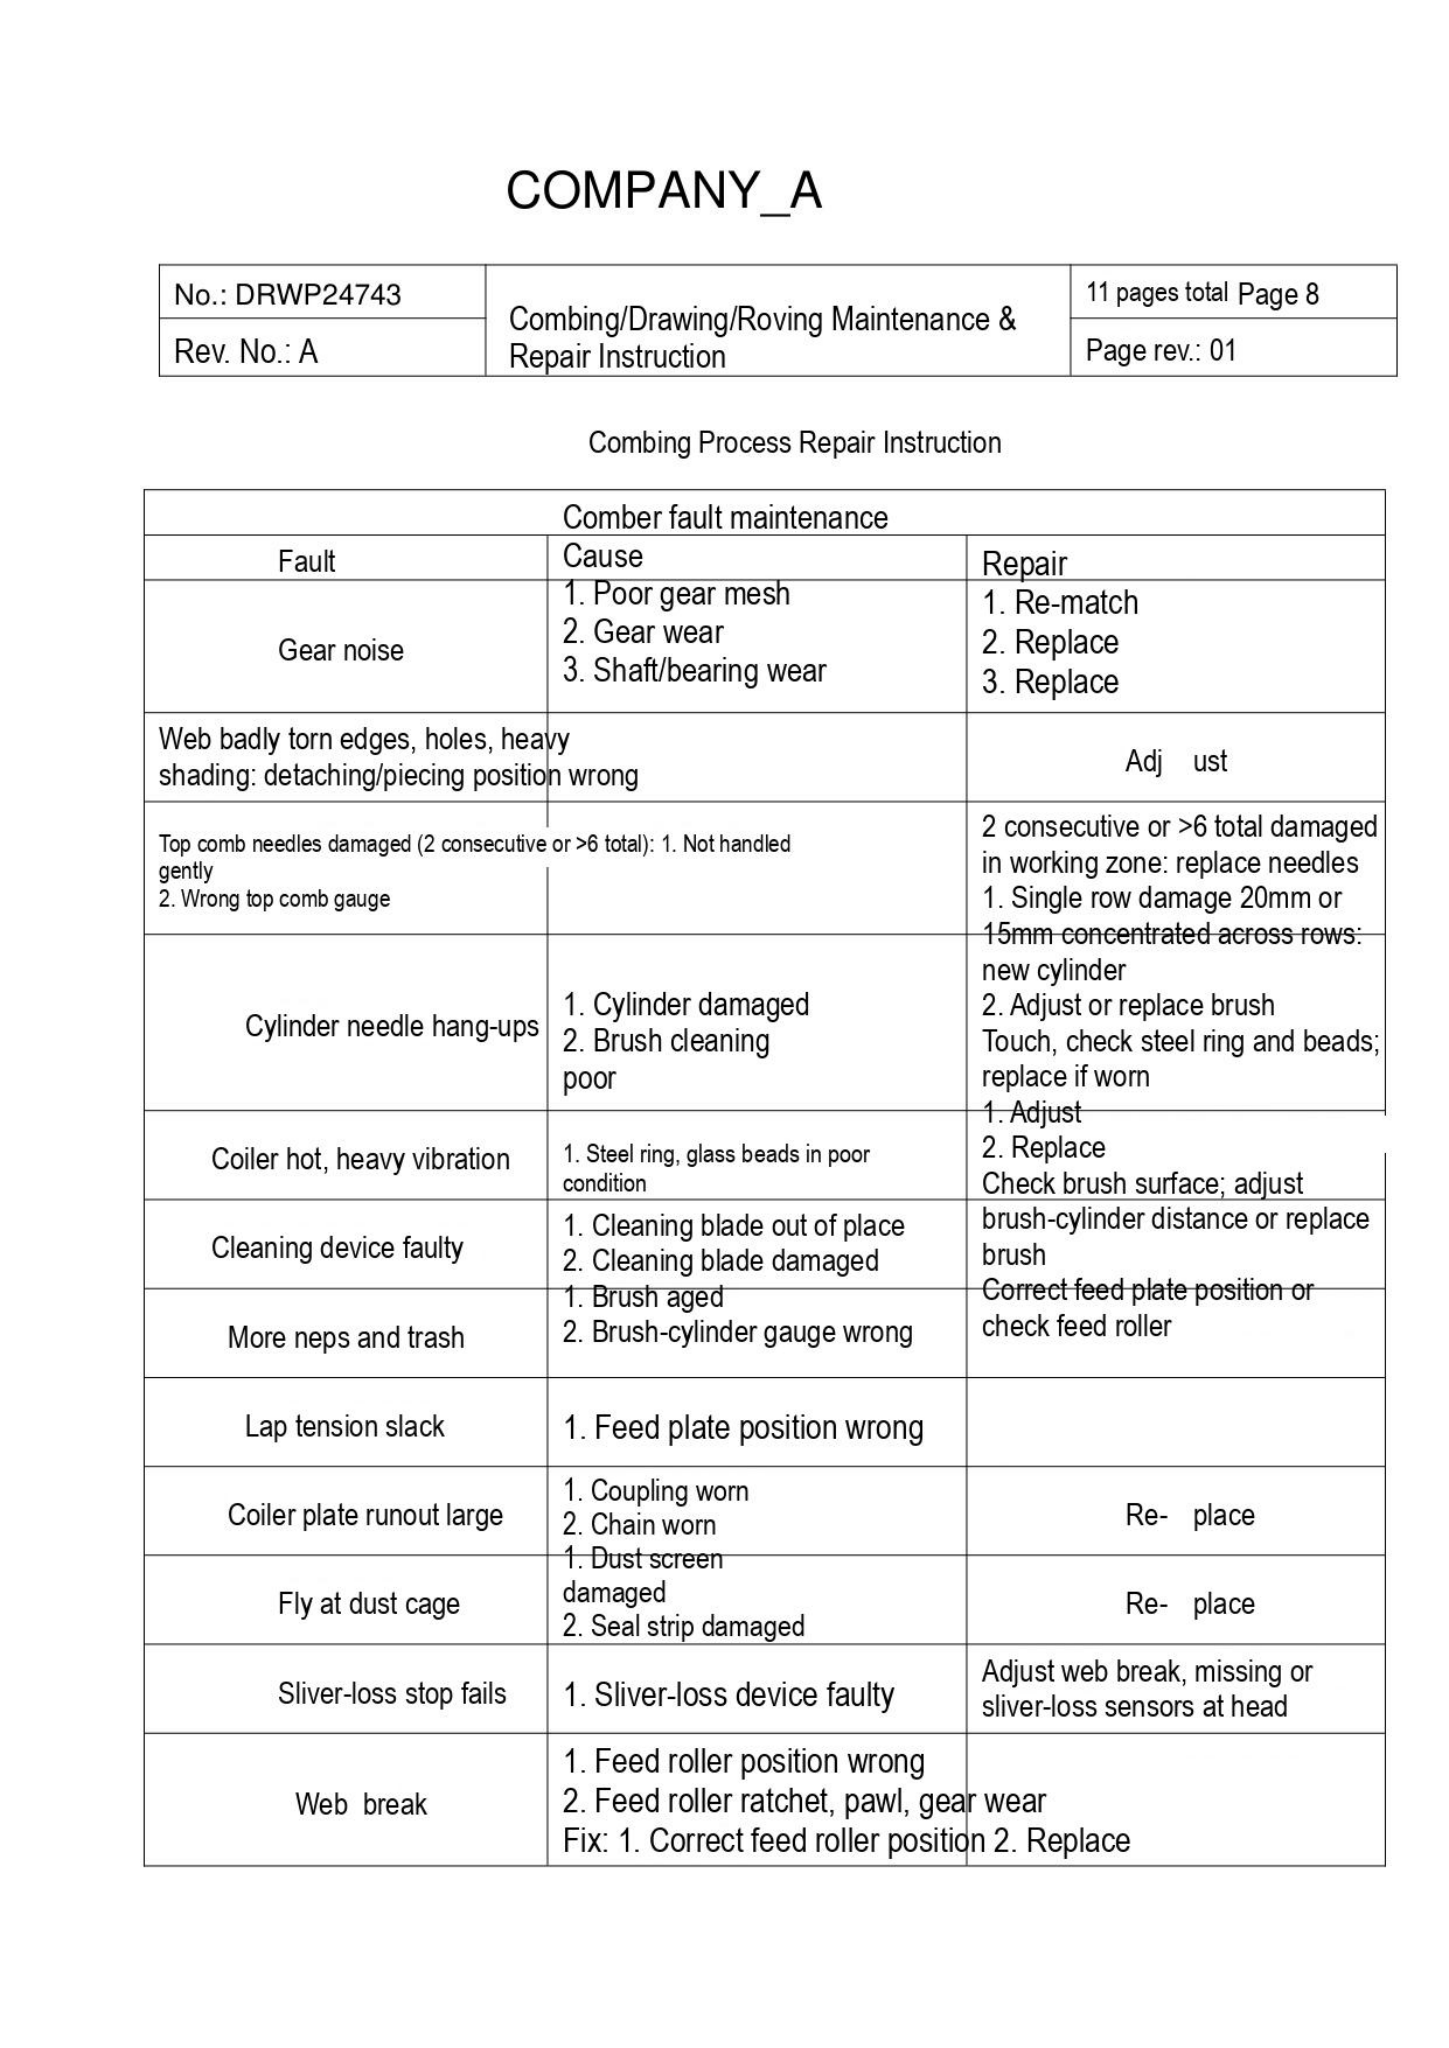COMPANY_A

| No.: DRWP24743 | Combing/Drawing/Roving Maintenance & Repair Instruction | 11 pages total Page 8 |
|---|---|---|
| Rev. No.: A | | Page rev.: 01 |

Combing Process Repair Instruction

| Comber fault maintenance | | |
|---|---|---|
| Fault | Cause | Repair |
| Gear noise | 1. Poor gear mesh<br>2. Gear wear<br>3. Shaft/bearing wear | 1. Re-match<br>2. Replace<br>3. Replace |
| Web badly torn edges, holes, heavy shading: detaching/piecing position wrong | | Adj ust |
| Top comb needles damaged (2 consecutive or >6 total): 1. Not handled gently<br>2. Wrong top comb gauge | | 2 consecutive or >6 total damaged in working zone: replace needles<br>1. Single row damage 20mm or |
| Cylinder needle hang-ups | 1. Cylinder damaged<br>2. Brush cleaning poor | 15mm concentrated across rows: new cylinder<br>2. Adjust or replace brush<br>Touch, check steel ring and beads; replace if worn |
| Coiler hot, heavy vibration | 1. Steel ring, glass beads in poor condition | 1. Adjust<br>2. Replace<br>Check brush surface; adjust |
| Cleaning device faulty | 1. Cleaning blade out of place<br>2. Cleaning blade damaged | brush-cylinder distance or replace brush |
| More neps and trash | 1. Brush aged<br>2. Brush-cylinder gauge wrong | Correct feed plate position or check feed roller |
| Lap tension slack | 1. Feed plate position wrong | |
| Coiler plate runout large | 1. Coupling worn<br>2. Chain worn | Re- place |
| Fly at dust cage | 1. Dust screen damaged<br>2. Seal strip damaged | Re- place |
| Sliver-loss stop fails | 1. Sliver-loss device faulty | Adjust web break, missing or sliver-loss sensors at head |
| Web break | 1. Feed roller position wrong<br>2. Feed roller ratchet, pawl, gear wear<br>Fix: 1. Correct feed roller position 2. Replace | |
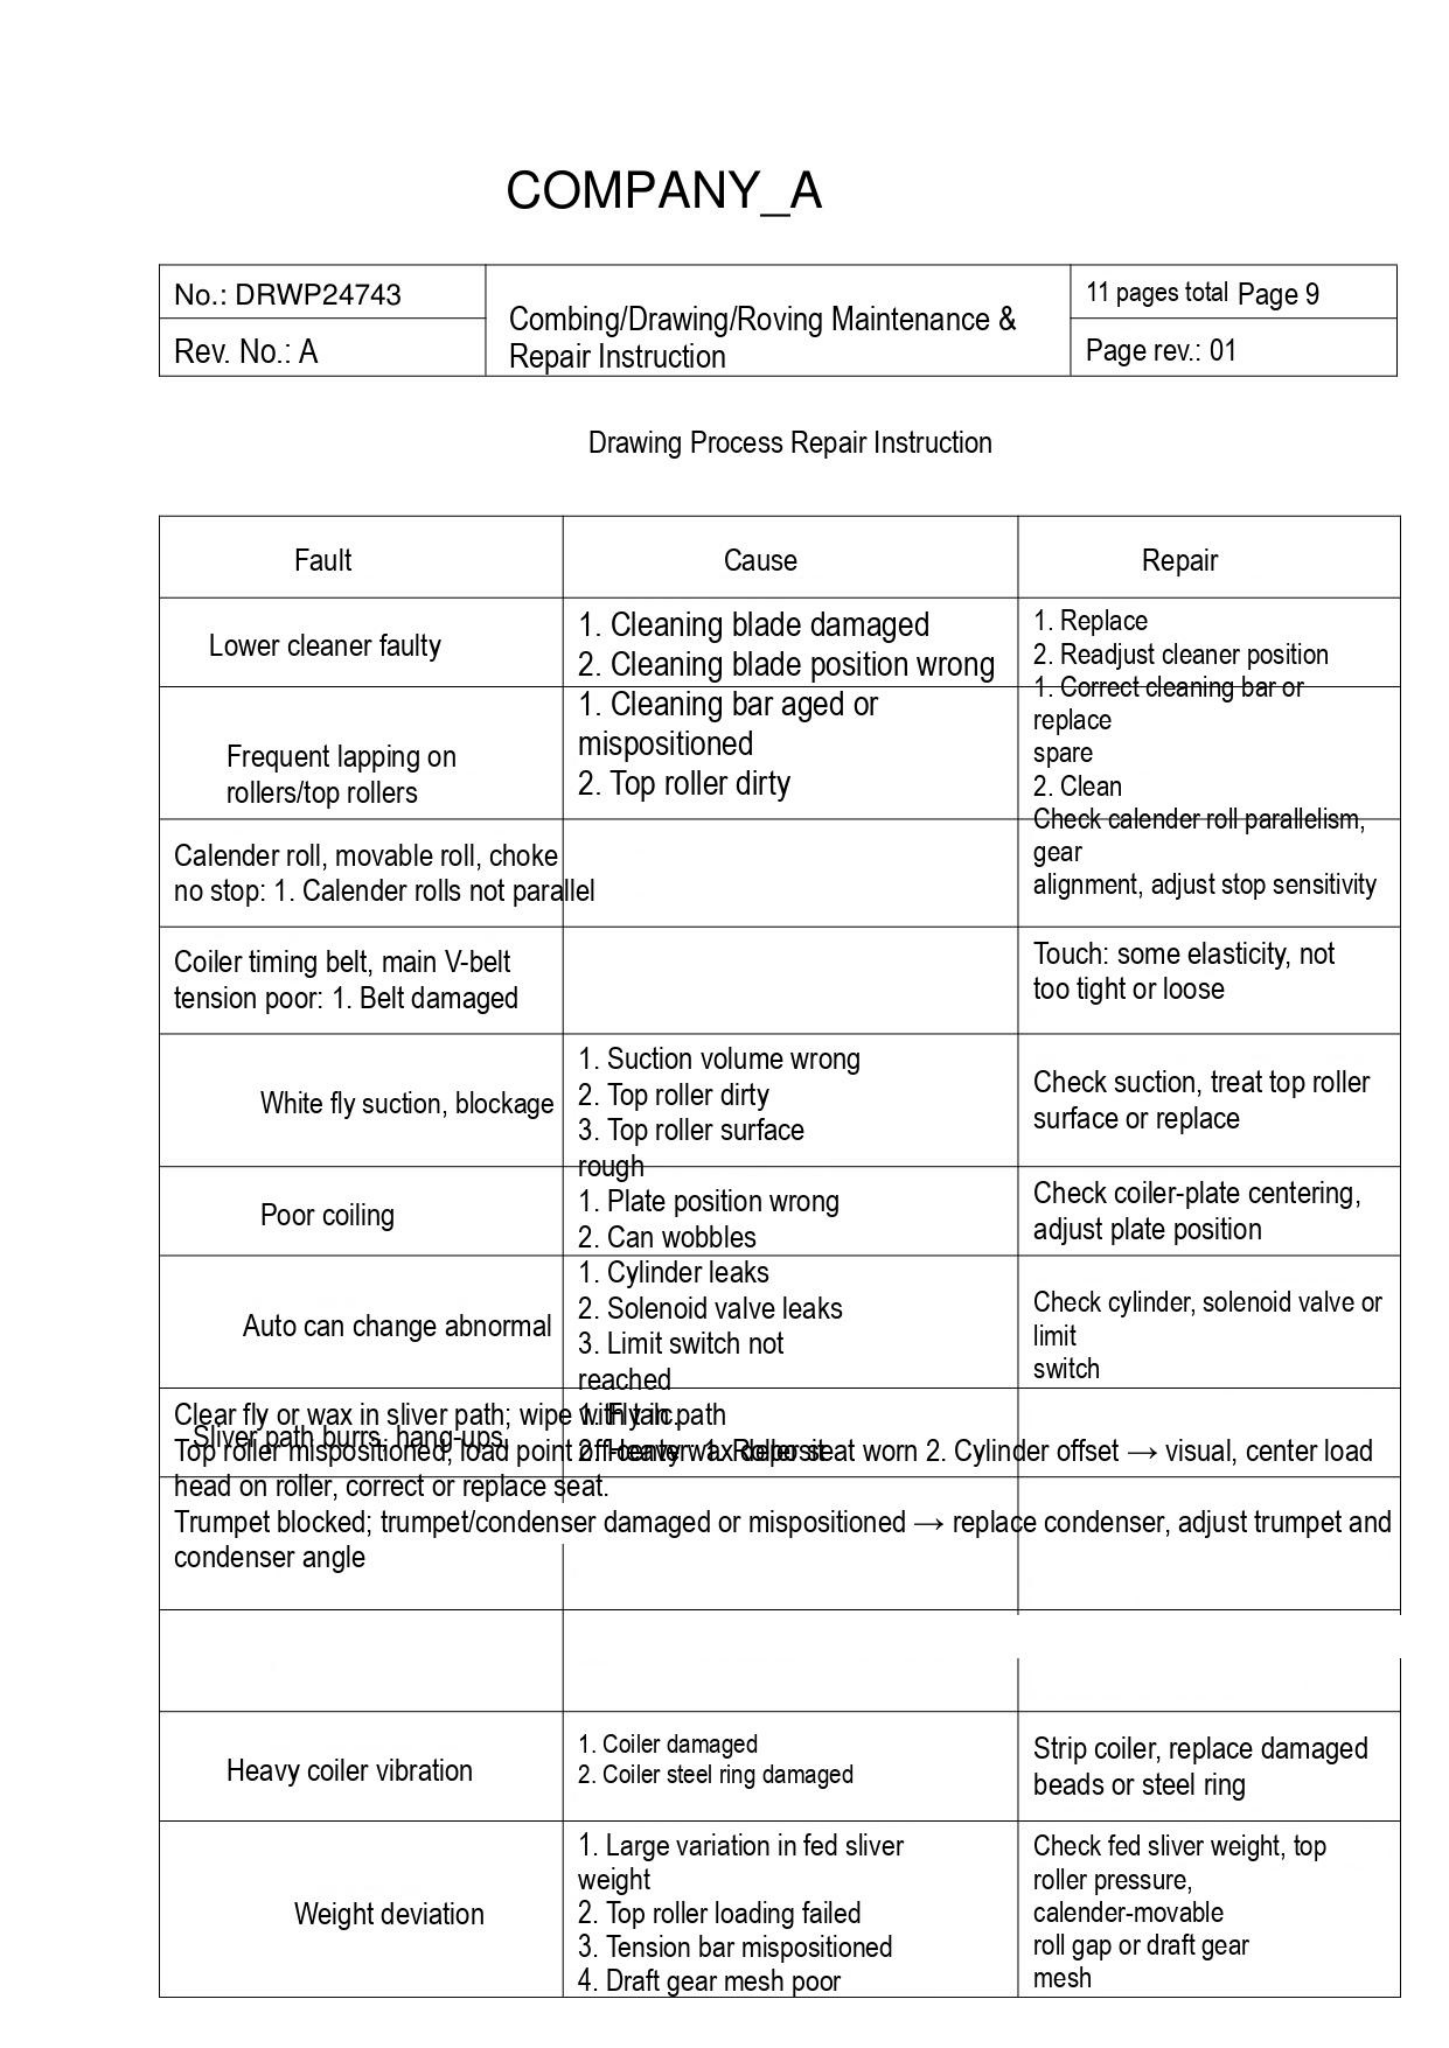# COMPANY_A

| No.: DRWP24743 | Combing/Drawing/Roving Maintenance & Repair Instruction | 11 pages total Page 9 |
|---|---|---|
| Rev. No.: A | | Page rev.: 01 |

Drawing Process Repair Instruction

| Fault | Cause | Repair |
|---|---|---|
| Lower cleaner faulty | 1. Cleaning blade damaged<br>2. Cleaning blade position wrong | 1. Replace<br>2. Readjust cleaner position |
| Frequent lapping on rollers/top rollers | 1. Cleaning bar aged or mispositioned<br>2. Top roller dirty | 1. Correct cleaning bar or replace spare<br>2. Clean |
| Calender roll, movable roll, choke no stop: 1. Calender rolls not parallel | | Check calender roll parallelism, gear alignment, adjust stop sensitivity |
| Coiler timing belt, main V-belt tension poor: 1. Belt damaged | | Touch: some elasticity, not too tight or loose |
| White fly suction, blockage | 1. Suction volume wrong<br>2. Top roller dirty<br>3. Top roller surface rough | Check suction, treat top roller surface or replace |
| Poor coiling | 1. Plate position wrong<br>2. Can wobbles | Check coiler-plate centering, adjust plate position |
| Auto can change abnormal | 1. Cylinder leaks<br>2. Solenoid valve leaks<br>3. Limit switch not reached | Check cylinder, solenoid valve or limit switch |
| Sliver path burrs, hang-ups | 1. Fly in path<br>2. Heavy wax deposit | Clear fly or wax in sliver path; wipe with talc. |
| Top roller mispositioned, load point off-center → 1. Roller seat worn 2. Cylinder offset → visual, center load head on roller, correct or replace seat.<br>Trumpet blocked; trumpet/condenser damaged or mispositioned → replace condenser, adjust trumpet and condenser angle | | |
| | | |
| Heavy coiler vibration | 1. Coiler damaged<br>2. Coiler steel ring damaged | Strip coiler, replace damaged beads or steel ring |
| Weight deviation | 1. Large variation in fed sliver weight<br>2. Top roller loading failed<br>3. Tension bar mispositioned<br>4. Draft gear mesh poor | Check fed sliver weight, top roller pressure, calender-movable roll gap or draft gear mesh |
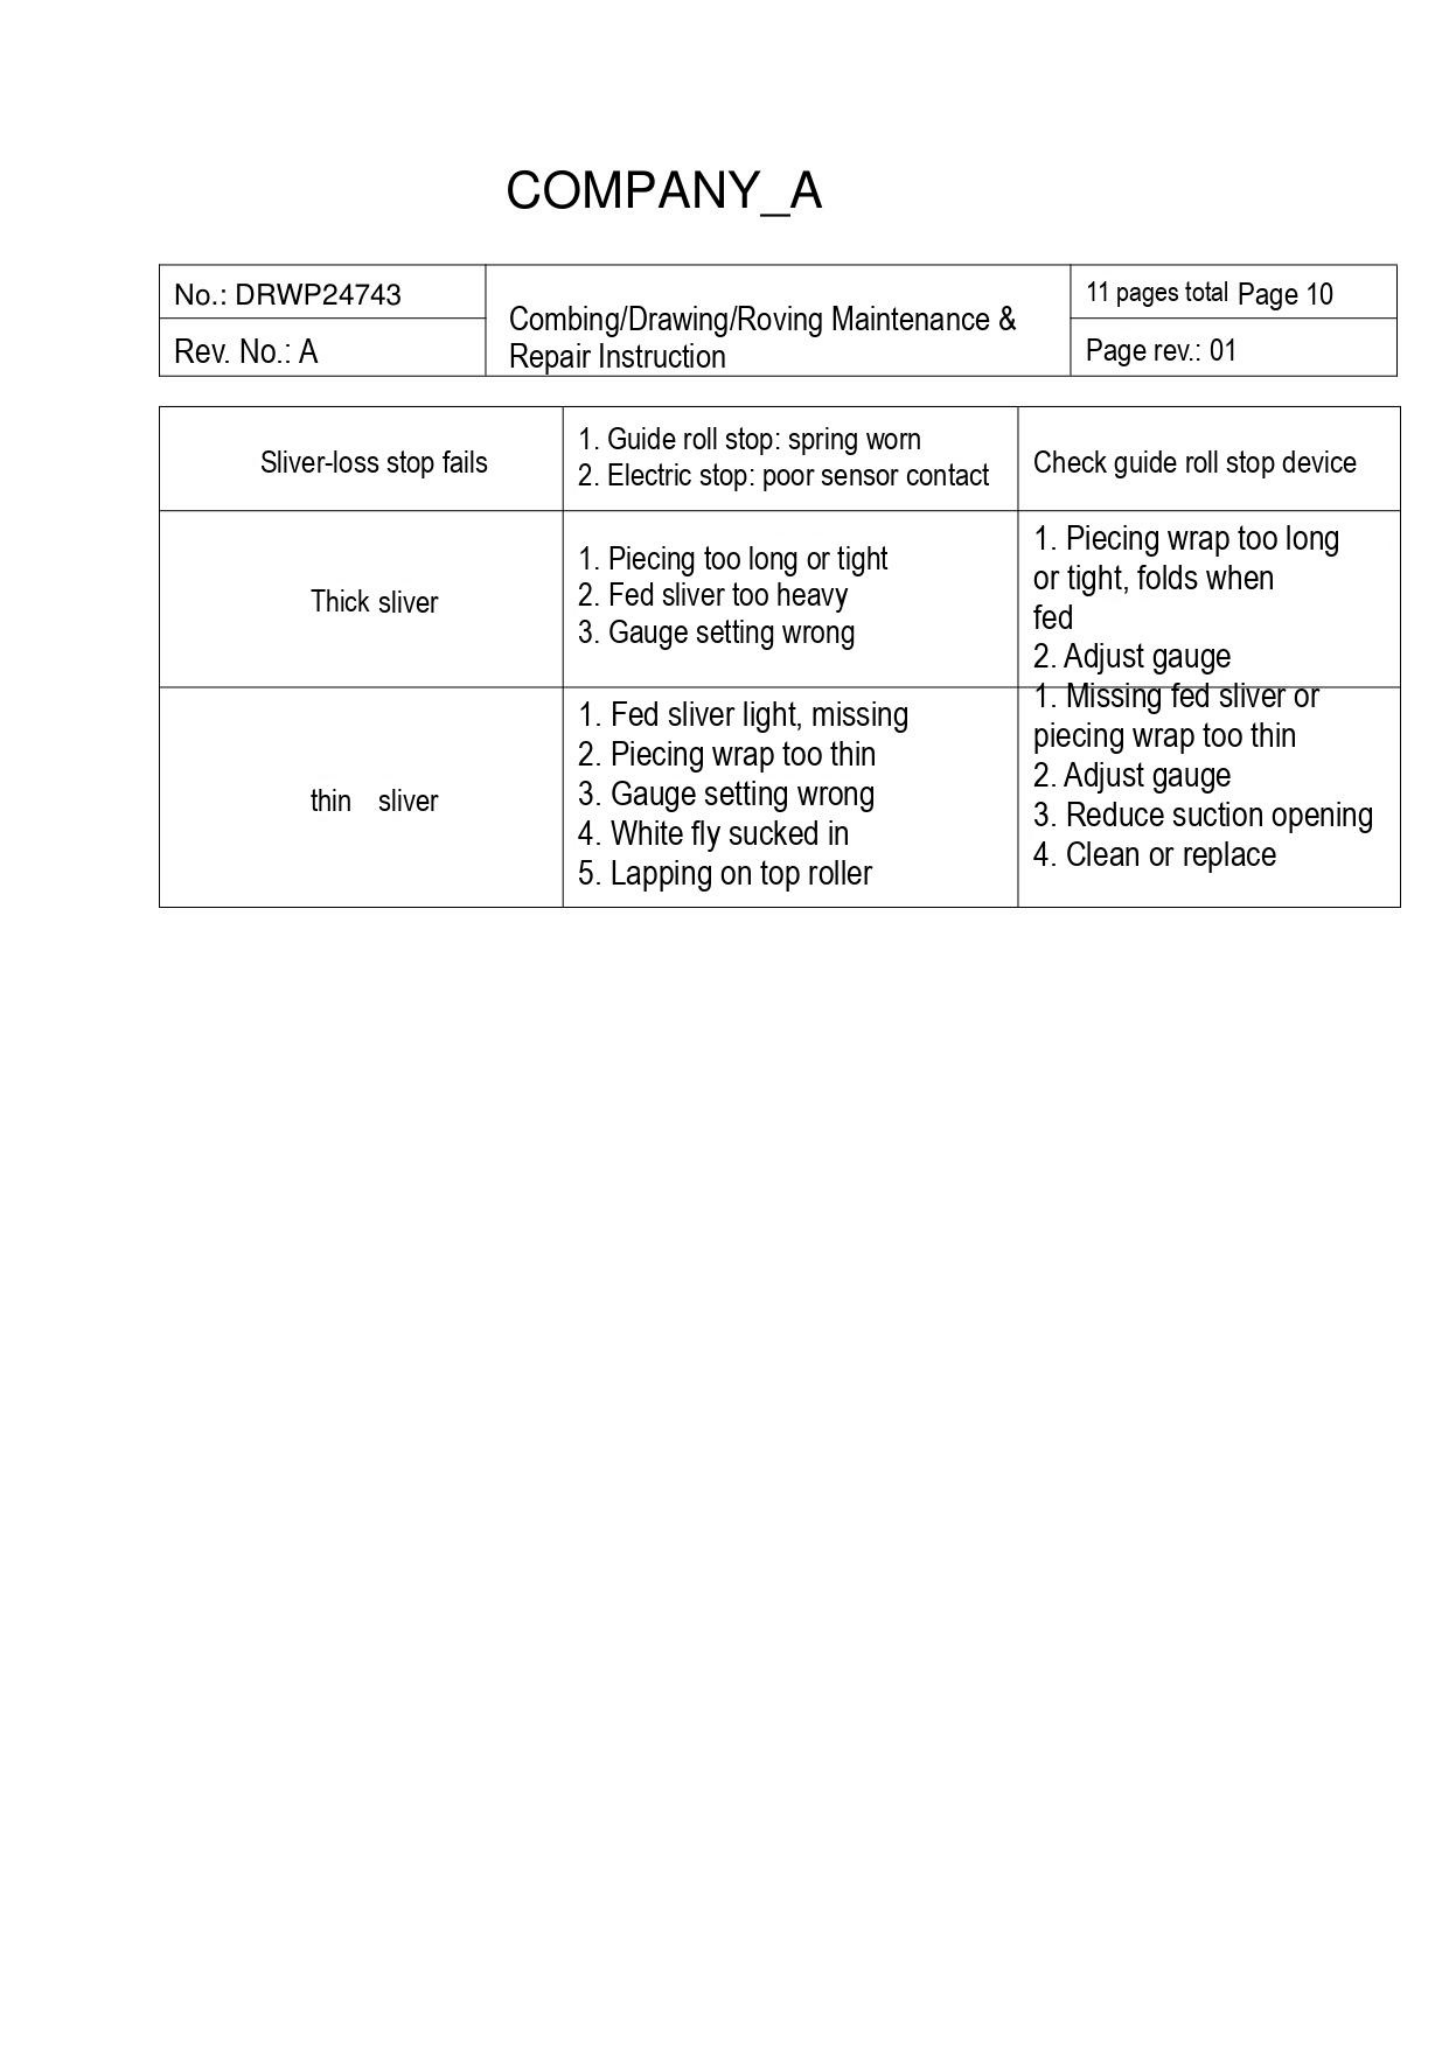COMPANY_A

| No.: DRWP24743 | Combing/Drawing/Roving Maintenance & Repair Instruction | 11 pages total Page 10 |
|---|---|---|
| Rev. No.: A | | Page rev.: 01 |

| Sliver-loss stop fails | 1. Guide roll stop: spring worn<br>2. Electric stop: poor sensor contact | Check guide roll stop device |
|---|---|---|
| Thick sliver | 1. Piecing too long or tight<br>2. Fed sliver too heavy<br>3. Gauge setting wrong | 1. Piecing wrap too long or tight, folds when fed<br>2. Adjust gauge |
| thin sliver | 1. Fed sliver light, missing<br>2. Piecing wrap too thin<br>3. Gauge setting wrong<br>4. White fly sucked in<br>5. Lapping on top roller | 1. Missing fed sliver or piecing wrap too thin<br>2. Adjust gauge<br>3. Reduce suction opening<br>4. Clean or replace |
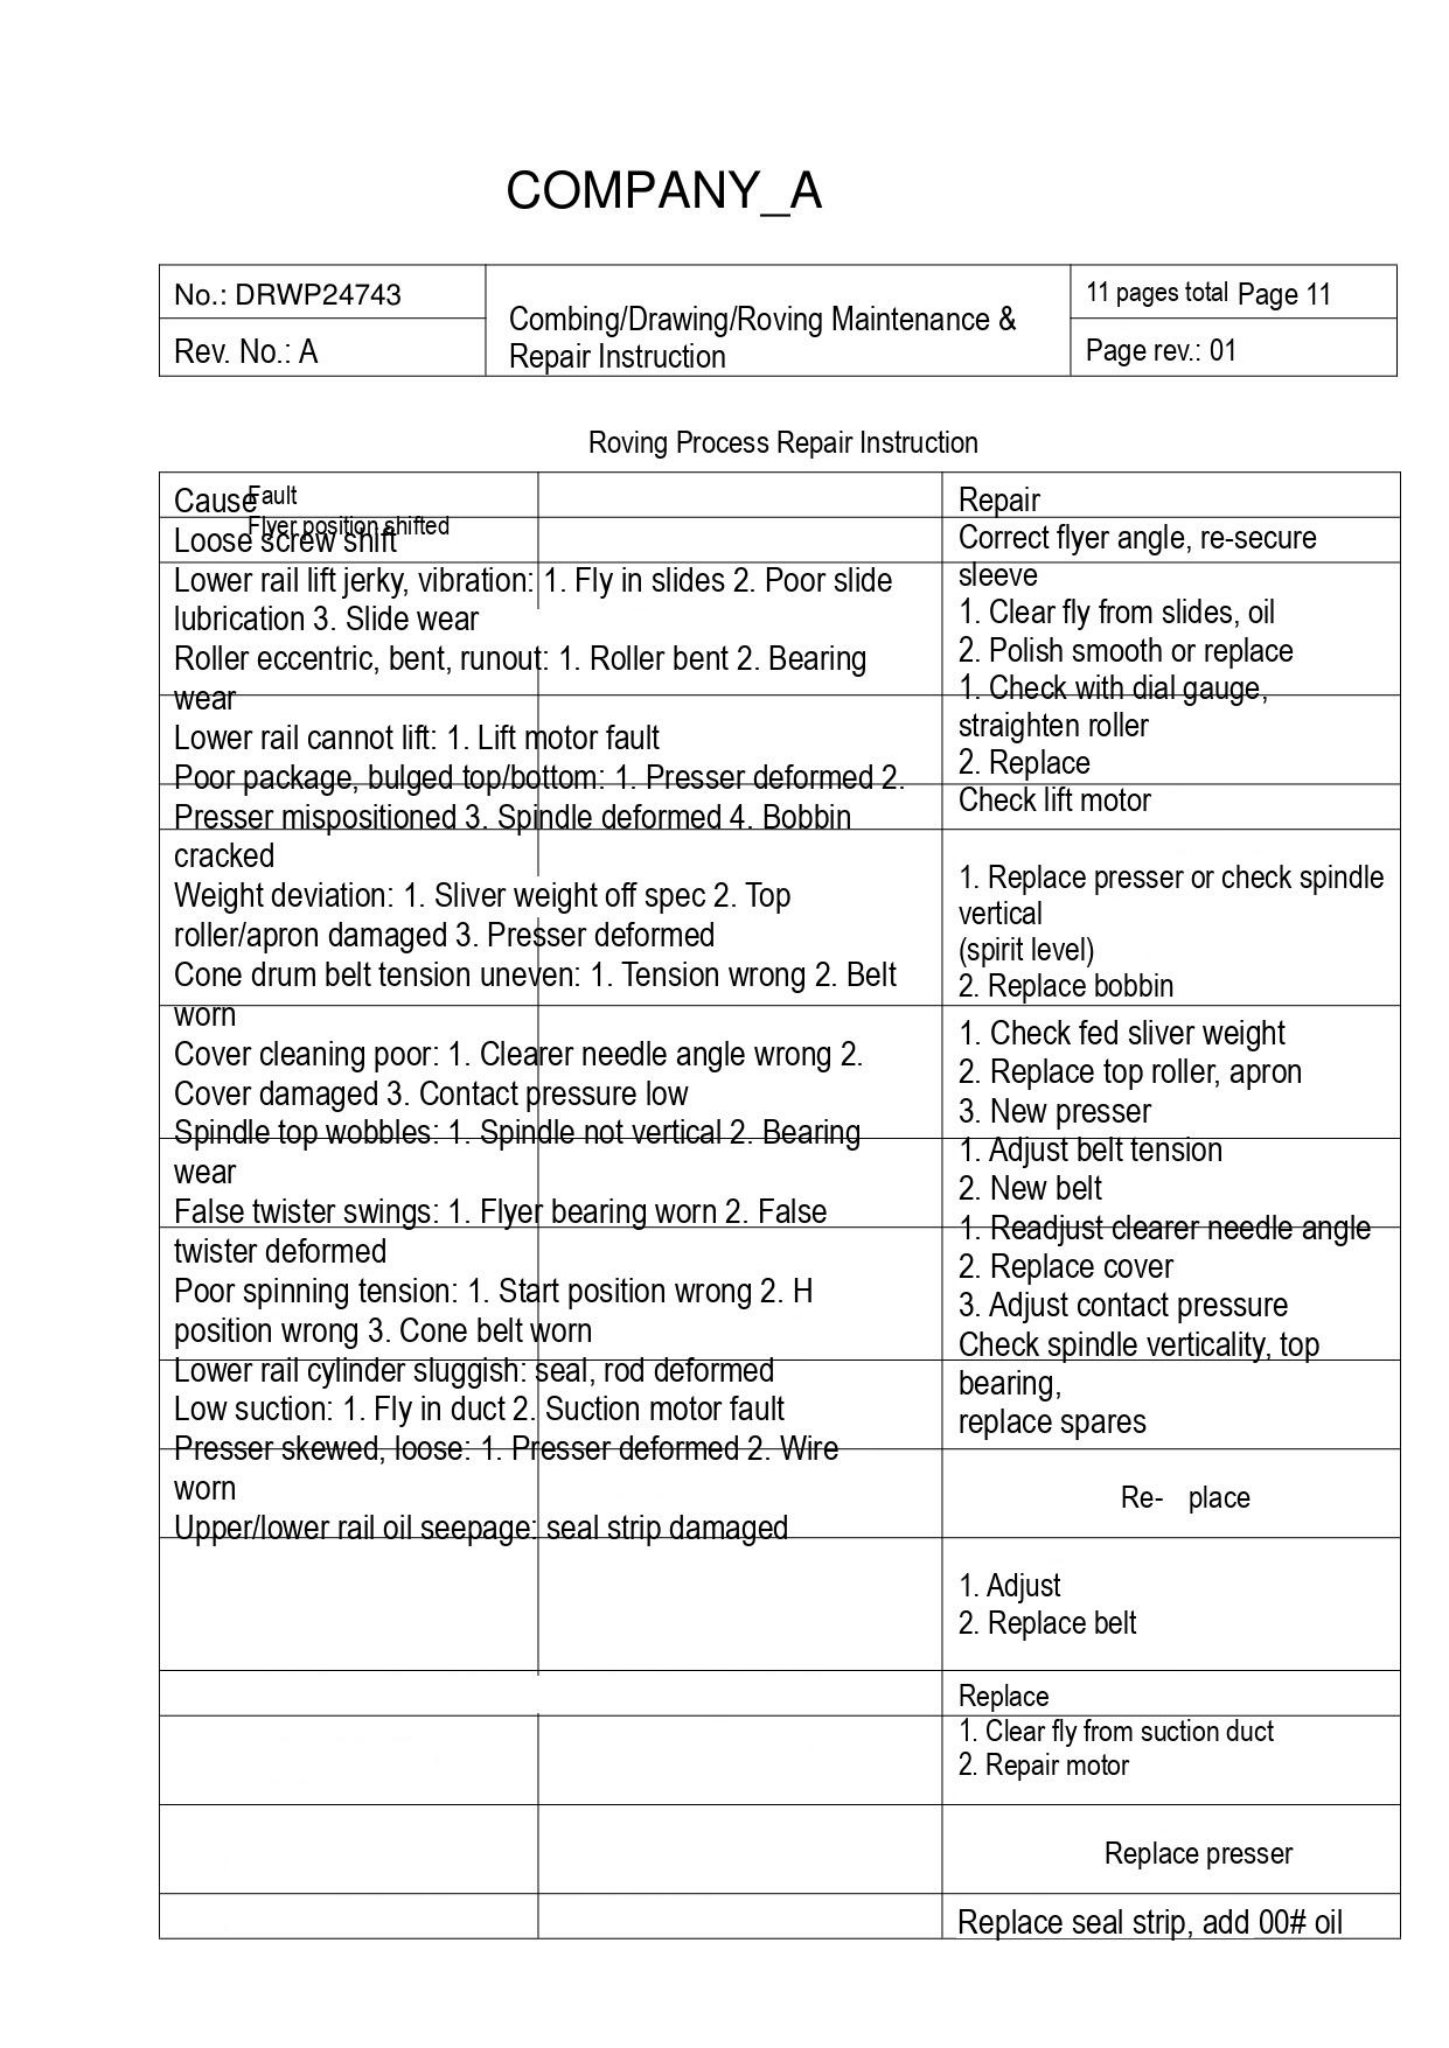COMPANY_A

| No.: DRWP24743 | Combing/Drawing/Roving Maintenance & Repair Instruction | 11 pages total Page 11 |
|---|---|---|
| Rev. No.: A | | Page rev.: 01 |

Roving Process Repair Instruction

| Cause Fault | | Repair |
|---|---|---|
| Loose screw shift Flyer position shifted | | Correct flyer angle, re-secure |
| Lower rail lift jerky, vibration: 1. Fly in slides 2. Poor slide lubrication 3. Slide wear<br>Roller eccentric, bent, runout: 1. Roller bent 2. Bearing | | sleeve<br>1. Clear fly from slides, oil<br>2. Polish smooth or replace |
| wear<br>Lower rail cannot lift: 1. Lift motor fault<br>Poor package, bulged top/bottom: 1. Presser deformed 2. | | 1. Check with dial gauge, straighten roller<br>2. Replace |
| Presser mispositioned 3. Spindle deformed 4. Bobbin | | Check lift motor |
| cracked<br>Weight deviation: 1. Sliver weight off spec 2. Top roller/apron damaged 3. Presser deformed<br>Cone drum belt tension uneven: 1. Tension wrong 2. Belt | | 1. Replace presser or check spindle vertical<br>(spirit level)<br>2. Replace bobbin |
| worn<br>Cover cleaning poor: 1. Clearer needle angle wrong 2. Cover damaged 3. Contact pressure low<br>Spindle top wobbles: 1. Spindle not vertical 2. Bearing | | 1. Check fed sliver weight<br>2. Replace top roller, apron<br>3. New presser |
| wear<br>False twister swings: 1. Flyer bearing worn 2. False | | 1. Adjust belt tension<br>2. New belt |
| twister deformed<br>Poor spinning tension: 1. Start position wrong 2. H position wrong 3. Cone belt worn | | 1. Readjust clearer needle angle<br>2. Replace cover<br>3. Adjust contact pressure<br>Check spindle verticality, top |
| Lower rail cylinder sluggish: seal, rod deformed<br>Low suction: 1. Fly in duct 2. Suction motor fault<br>Presser skewed, loose: 1. Presser deformed 2. Wire | | bearing,<br>replace spares |
| worn<br>Upper/lower rail oil seepage: seal strip damaged | | Re- place |
| | | 1. Adjust<br>2. Replace belt |
| | | Replace |
| | | 1. Clear fly from suction duct<br>2. Repair motor |
| | | Replace presser |
| | | Replace seal strip, add 00# oil |